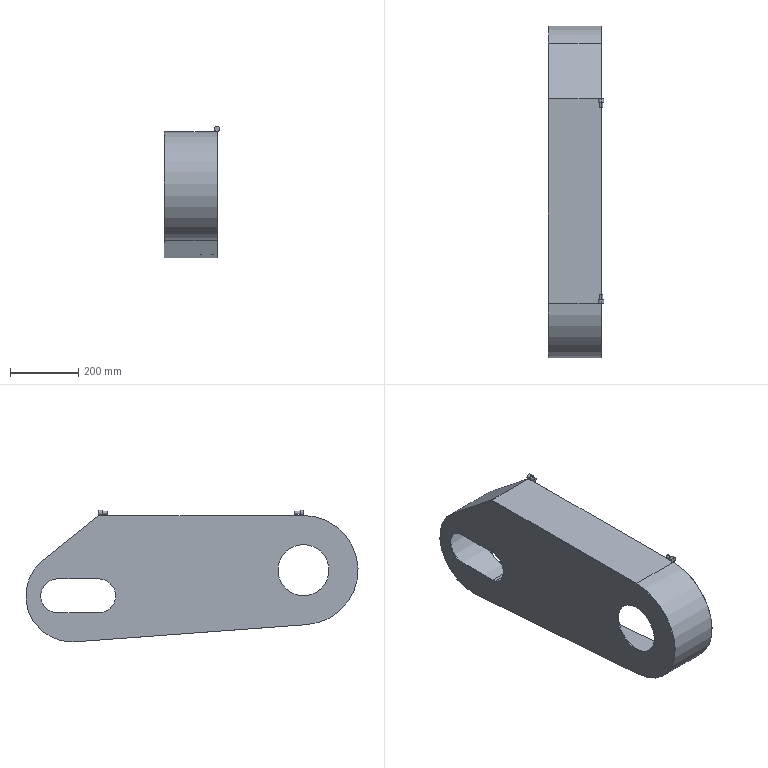Part | SolidWorks | features ICE 7, Extrusion 1, HoleWzd 1, WeldBeadFeat 1, WeldmentFeature 1 | 6 solids | 52 faces | box 163 x 973.632 x 386.5 mm | volume 1244808 mm3 | cylinder 29 | plane 23 | commonest cylinder face diameters 4.2 x8 10 x4 16 x4 270 x4 100 x2 150 x2
STEP:
#1=CARTESIAN_POINT('',(-160.,-325.,-45.));
#2=VERTEX_POINT('',#1);
#3=CARTESIAN_POINT('',(-160.,-325.,105.));
#4=VERTEX_POINT('',#3);
#5=CARTESIAN_POINT('',(-160.,-325.,30.));
#6=DIRECTION('',(-1.,0.,0.));
#7=DIRECTION('',(0.,0.,1.));
#8=AXIS2_PLACEMENT_3D('',#5,#6,#7);
#9=CIRCLE('',#8,75.);
#10=EDGE_CURVE('',#2,#4,#9,.T.);
#11=ORIENTED_EDGE('',*,*,#10,.T.);
#12=CARTESIAN_POINT('',(-158.,-325.,105.));
#13=VERTEX_POINT('',#12);
#14=CARTESIAN_POINT('',(-160.,-325.,105.));
#15=DIRECTION('',(1.,0.,0.));
#16=VECTOR('',#15,1000.);
#17=LINE('',#14,#16);
#18=EDGE_CURVE('',#4,#13,#17,.T.);
#19=ORIENTED_EDGE('',*,*,#18,.T.);
#20=CARTESIAN_POINT('',(-158.,-325.,-45.));
#21=VERTEX_POINT('',#20);
#22=CARTESIAN_POINT('',(-158.,-325.,30.));
#23=DIRECTION('',(-1.,0.,0.));
#24=DIRECTION('',(0.,0.,1.));
#25=AXIS2_PLACEMENT_3D('',#22,#23,#24);
#26=CIRCLE('',#25,75.);
#27=EDGE_CURVE('',#21,#13,#26,.T.);
#28=ORIENTED_EDGE('',*,*,#27,.F.);
#29=CARTESIAN_POINT('',(-160.,-325.,-45.));
#30=DIRECTION('',(1.,0.,0.));
#31=VECTOR('',#30,1000.);
#32=LINE('',#29,#31);
#33=EDGE_CURVE('',#2,#21,#32,.T.);
#34=ORIENTED_EDGE('',*,*,#33,.F.);
#35=EDGE_LOOP('',(#11,#19,#28,#34));
#36=FACE_OUTER_BOUND('',#35,.T.);
#37=CARTESIAN_POINT('',(-160.,-325.,30.));
#38=DIRECTION('',(1.,0.,0.));
#39=DIRECTION('',(0.,0.,-1.));
#40=AXIS2_PLACEMENT_3D('',#37,#38,#39);
#41=CYLINDRICAL_SURFACE('',#40,75.);
#42=ADVANCED_FACE('',(#36),#41,.F.);
#43=CARTESIAN_POINT('',(-160.,353.632,-180.5));
#44=VERTEX_POINT('',#43);
#45=CARTESIAN_POINT('',(-160.,343.627,-180.129));
#46=VERTEX_POINT('',#45);
#47=CARTESIAN_POINT('',(-160.,353.632,-45.5));
#48=DIRECTION('',(-1.,0.,0.));
#49=DIRECTION('',(0.,0.,1.));
#50=AXIS2_PLACEMENT_3D('',#47,#48,#49);
#51=CIRCLE('',#50,135.);
#52=EDGE_CURVE('',#44,#46,#51,.T.);
#53=ORIENTED_EDGE('',*,*,#52,.F.);
#54=CARTESIAN_POINT('',(-158.,353.632,-180.5));
#55=VERTEX_POINT('',#54);
#56=CARTESIAN_POINT('',(-160.,353.632,-180.5));
#57=DIRECTION('',(1.,0.,0.));
#58=VECTOR('',#57,1000.);
#59=LINE('',#56,#58);
#60=EDGE_CURVE('',#44,#55,#59,.T.);
#61=ORIENTED_EDGE('',*,*,#60,.T.);
#62=CARTESIAN_POINT('',(-158.,343.627,-180.129));
#63=VERTEX_POINT('',#62);
#64=CARTESIAN_POINT('',(-158.,353.632,-45.5));
#65=DIRECTION('',(-1.,0.,0.));
#66=DIRECTION('',(0.,0.,1.));
#67=AXIS2_PLACEMENT_3D('',#64,#65,#66);
#68=CIRCLE('',#67,135.);
#69=EDGE_CURVE('',#55,#63,#68,.T.);
#70=ORIENTED_EDGE('',*,*,#69,.T.);
#71=CARTESIAN_POINT('',(-160.,343.627,-180.129));
#72=DIRECTION('',(1.,0.,0.));
#73=VECTOR('',#72,1000.);
#74=LINE('',#71,#73);
#75=EDGE_CURVE('',#46,#63,#74,.T.);
#76=ORIENTED_EDGE('',*,*,#75,.F.);
#77=EDGE_LOOP('',(#53,#61,#70,#76));
#78=FACE_OUTER_BOUND('',#77,.T.);
#79=CARTESIAN_POINT('',(-160.,353.632,-45.5));
#80=DIRECTION('',(1.,0.,0.));
#81=DIRECTION('',(0.,0.,-1.));
#82=AXIS2_PLACEMENT_3D('',#79,#80,#81);
#83=CYLINDRICAL_SURFACE('',#82,135.);
#84=ADVANCED_FACE('',(#78),#83,.T.);
#85=CARTESIAN_POINT('',(-160.,-336.857,-129.56));
#86=VERTEX_POINT('',#85);
#87=CARTESIAN_POINT('',(-160.,-325.,190.));
#88=VERTEX_POINT('',#87);
#89=CARTESIAN_POINT('',(-160.,-325.,30.));
#90=DIRECTION('',(-1.,0.,0.));
#91=DIRECTION('',(0.,0.,1.));
#92=AXIS2_PLACEMENT_3D('',#89,#90,#91);
#93=CIRCLE('',#92,160.);
#94=EDGE_CURVE('',#86,#88,#93,.T.);
#95=ORIENTED_EDGE('',*,*,#94,.T.);
#96=CARTESIAN_POINT('',(-160.,275.,190.));
#97=VERTEX_POINT('',#96);
#98=CARTESIAN_POINT('',(-160.,-325.,190.));
#99=DIRECTION('',(0.,1.,0.));
#100=VECTOR('',#99,1000.);
#101=LINE('',#98,#100);
#102=EDGE_CURVE('',#88,#97,#101,.T.);
#103=ORIENTED_EDGE('',*,*,#102,.T.);
#104=CARTESIAN_POINT('',(-160.,437.851,60.009));
#105=VERTEX_POINT('',#104);
#106=CARTESIAN_POINT('',(-160.,275.,190.));
#107=DIRECTION('',(0.,0.7815,-0.6238));
#108=VECTOR('',#107,1000.);
#109=LINE('',#106,#108);
#110=EDGE_CURVE('',#97,#105,#109,.T.);
#111=ORIENTED_EDGE('',*,*,#110,.T.);
#112=CARTESIAN_POINT('',(-160.,353.632,-45.5));
#113=DIRECTION('',(-1.,0.,0.));
#114=DIRECTION('',(0.,0.,1.));
#115=AXIS2_PLACEMENT_3D('',#112,#113,#114);
#116=CIRCLE('',#115,135.);
#117=EDGE_CURVE('',#105,#44,#116,.T.);
#118=ORIENTED_EDGE('',*,*,#117,.T.);
#119=ORIENTED_EDGE('',*,*,#52,.T.);
#120=CARTESIAN_POINT('',(-160.,343.627,-180.129));
#121=DIRECTION('',(0.,-0.9973,0.07411));
#122=VECTOR('',#121,1000.);
#123=LINE('',#120,#122);
#124=EDGE_CURVE('',#46,#86,#123,.T.);
#125=ORIENTED_EDGE('',*,*,#124,.T.);
#126=EDGE_LOOP('',(#95,#103,#111,#118,#119,#125));
#127=FACE_OUTER_BOUND('',#126,.T.);
#128=ORIENTED_EDGE('',*,*,#10,.F.);
#129=CARTESIAN_POINT('',(-160.,-325.,30.));
#130=DIRECTION('',(-1.,0.,0.));
#131=DIRECTION('',(0.,0.,1.));
#132=AXIS2_PLACEMENT_3D('',#129,#130,#131);
#133=CIRCLE('',#132,75.);
#134=EDGE_CURVE('',#4,#2,#133,.T.);
#135=ORIENTED_EDGE('',*,*,#134,.F.);
#136=EDGE_LOOP('',(#128,#135));
#137=FACE_BOUND('',#136,.T.);
#138=CARTESIAN_POINT('',(-160.,395.,-95.5));
#139=VERTEX_POINT('',#138);
#140=CARTESIAN_POINT('',(-160.,275.,-95.5));
#141=VERTEX_POINT('',#140);
#142=CARTESIAN_POINT('',(-160.,395.,-95.5));
#143=DIRECTION('',(0.,-1.,0.));
#144=VECTOR('',#143,1000.);
#145=LINE('',#142,#144);
#146=EDGE_CURVE('',#139,#141,#145,.T.);
#147=ORIENTED_EDGE('',*,*,#146,.F.);
#148=CARTESIAN_POINT('',(-160.,395.,4.5));
#149=VERTEX_POINT('',#148);
#150=CARTESIAN_POINT('',(-160.,395.,-45.5));
#151=DIRECTION('',(-1.,0.,0.));
#152=DIRECTION('',(0.,0.,1.));
#153=AXIS2_PLACEMENT_3D('',#150,#151,#152);
#154=CIRCLE('',#153,50.);
#155=EDGE_CURVE('',#149,#139,#154,.T.);
#156=ORIENTED_EDGE('',*,*,#155,.F.);
#157=CARTESIAN_POINT('',(-160.,275.,4.5));
#158=VERTEX_POINT('',#157);
#159=CARTESIAN_POINT('',(-160.,395.,4.5));
#160=DIRECTION('',(0.,1.,0.));
#161=VECTOR('',#160,1000.);
#162=LINE('',#159,#161);
#163=EDGE_CURVE('',#158,#149,#162,.T.);
#164=ORIENTED_EDGE('',*,*,#163,.F.);
#165=CARTESIAN_POINT('',(-160.,275.,-45.5));
#166=DIRECTION('',(-1.,0.,0.));
#167=DIRECTION('',(0.,0.,1.));
#168=AXIS2_PLACEMENT_3D('',#165,#166,#167);
#169=CIRCLE('',#168,50.);
#170=EDGE_CURVE('',#141,#158,#169,.T.);
#171=ORIENTED_EDGE('',*,*,#170,.F.);
#172=EDGE_LOOP('',(#147,#156,#164,#171));
#173=FACE_BOUND('',#172,.T.);
#174=CARTESIAN_POINT('',(-160.,-325.,30.));
#175=DIRECTION('',(-1.,0.,0.));
#176=DIRECTION('',(0.,0.,1.));
#177=AXIS2_PLACEMENT_3D('',#174,#175,#176);
#178=PLANE('',#177);
#179=ADVANCED_FACE('',(#127,#137,#173),#178,.T.);
#180=ORIENTED_EDGE('',*,*,#27,.T.);
#181=CARTESIAN_POINT('',(-158.,-325.,30.));
#182=DIRECTION('',(-1.,0.,0.));
#183=DIRECTION('',(0.,0.,1.));
#184=AXIS2_PLACEMENT_3D('',#181,#182,#183);
#185=CIRCLE('',#184,75.);
#186=EDGE_CURVE('',#13,#21,#185,.T.);
#187=ORIENTED_EDGE('',*,*,#186,.T.);
#188=EDGE_LOOP('',(#180,#187));
#189=FACE_BOUND('',#188,.T.);
#190=CARTESIAN_POINT('',(-158.,-336.857,-129.56));
#191=VERTEX_POINT('',#190);
#192=CARTESIAN_POINT('',(-158.,-325.,190.));
#193=VERTEX_POINT('',#192);
#194=CARTESIAN_POINT('',(-158.,-325.,30.));
#195=DIRECTION('',(-1.,0.,0.));
#196=DIRECTION('',(0.,0.,1.));
#197=AXIS2_PLACEMENT_3D('',#194,#195,#196);
#198=CIRCLE('',#197,160.);
#199=EDGE_CURVE('',#191,#193,#198,.T.);
#200=ORIENTED_EDGE('',*,*,#199,.F.);
#201=CARTESIAN_POINT('',(-158.,343.627,-180.129));
#202=DIRECTION('',(0.,-0.9973,0.07411));
#203=VECTOR('',#202,1000.);
#204=LINE('',#201,#203);
#205=EDGE_CURVE('',#63,#191,#204,.T.);
#206=ORIENTED_EDGE('',*,*,#205,.F.);
#207=ORIENTED_EDGE('',*,*,#69,.F.);
#208=CARTESIAN_POINT('',(-158.,437.851,60.009));
#209=VERTEX_POINT('',#208);
#210=CARTESIAN_POINT('',(-158.,353.632,-45.5));
#211=DIRECTION('',(-1.,0.,0.));
#212=DIRECTION('',(0.,0.,1.));
#213=AXIS2_PLACEMENT_3D('',#210,#211,#212);
#214=CIRCLE('',#213,135.);
#215=EDGE_CURVE('',#209,#55,#214,.T.);
#216=ORIENTED_EDGE('',*,*,#215,.F.);
#217=CARTESIAN_POINT('',(-158.,275.,190.));
#218=VERTEX_POINT('',#217);
#219=CARTESIAN_POINT('',(-158.,275.,190.));
#220=DIRECTION('',(0.,0.7815,-0.6238));
#221=VECTOR('',#220,1000.);
#222=LINE('',#219,#221);
#223=EDGE_CURVE('',#218,#209,#222,.T.);
#224=ORIENTED_EDGE('',*,*,#223,.F.);
#225=CARTESIAN_POINT('',(-158.,-325.,190.));
#226=DIRECTION('',(0.,1.,0.));
#227=VECTOR('',#226,1000.);
#228=LINE('',#225,#227);
#229=EDGE_CURVE('',#193,#218,#228,.T.);
#230=ORIENTED_EDGE('',*,*,#229,.F.);
#231=EDGE_LOOP('',(#200,#206,#207,#216,#224,#230));
#232=FACE_OUTER_BOUND('',#231,.T.);
#233=CARTESIAN_POINT('',(-158.,395.,4.5));
#234=VERTEX_POINT('',#233);
#235=CARTESIAN_POINT('',(-158.,395.,-95.5));
#236=VERTEX_POINT('',#235);
#237=CARTESIAN_POINT('',(-158.,395.,-45.5));
#238=DIRECTION('',(-1.,0.,0.));
#239=DIRECTION('',(0.,0.,1.));
#240=AXIS2_PLACEMENT_3D('',#237,#238,#239);
#241=CIRCLE('',#240,50.);
#242=EDGE_CURVE('',#234,#236,#241,.T.);
#243=ORIENTED_EDGE('',*,*,#242,.T.);
#244=CARTESIAN_POINT('',(-158.,275.,-95.5));
#245=VERTEX_POINT('',#244);
#246=CARTESIAN_POINT('',(-158.,395.,-95.5));
#247=DIRECTION('',(0.,-1.,0.));
#248=VECTOR('',#247,1000.);
#249=LINE('',#246,#248);
#250=EDGE_CURVE('',#236,#245,#249,.T.);
#251=ORIENTED_EDGE('',*,*,#250,.T.);
#252=CARTESIAN_POINT('',(-158.,275.,4.5));
#253=VERTEX_POINT('',#252);
#254=CARTESIAN_POINT('',(-158.,275.,-45.5));
#255=DIRECTION('',(-1.,0.,0.));
#256=DIRECTION('',(0.,0.,1.));
#257=AXIS2_PLACEMENT_3D('',#254,#255,#256);
#258=CIRCLE('',#257,50.);
#259=EDGE_CURVE('',#245,#253,#258,.T.);
#260=ORIENTED_EDGE('',*,*,#259,.T.);
#261=CARTESIAN_POINT('',(-158.,395.,4.5));
#262=DIRECTION('',(0.,1.,0.));
#263=VECTOR('',#262,1000.);
#264=LINE('',#261,#263);
#265=EDGE_CURVE('',#253,#234,#264,.T.);
#266=ORIENTED_EDGE('',*,*,#265,.T.);
#267=EDGE_LOOP('',(#243,#251,#260,#266));
#268=FACE_BOUND('',#267,.T.);
#269=CARTESIAN_POINT('',(-158.,-325.,30.));
#270=DIRECTION('',(-1.,0.,0.));
#271=DIRECTION('',(0.,0.,1.));
#272=AXIS2_PLACEMENT_3D('',#269,#270,#271);
#273=PLANE('',#272);
#274=ADVANCED_FACE('',(#189,#232,#268),#273,.F.);
#275=ORIENTED_EDGE('',*,*,#199,.T.);
#276=CARTESIAN_POINT('',(-160.,-325.,190.));
#277=DIRECTION('',(1.,0.,0.));
#278=VECTOR('',#277,1000.);
#279=LINE('',#276,#278);
#280=EDGE_CURVE('',#88,#193,#279,.T.);
#281=ORIENTED_EDGE('',*,*,#280,.F.);
#282=ORIENTED_EDGE('',*,*,#94,.F.);
#283=CARTESIAN_POINT('',(-160.,-336.857,-129.56));
#284=DIRECTION('',(1.,0.,0.));
#285=VECTOR('',#284,1000.);
#286=LINE('',#283,#285);
#287=EDGE_CURVE('',#86,#191,#286,.T.);
#288=ORIENTED_EDGE('',*,*,#287,.T.);
#289=EDGE_LOOP('',(#275,#281,#282,#288));
#290=FACE_OUTER_BOUND('',#289,.T.);
#291=CARTESIAN_POINT('',(-160.,-325.,30.));
#292=DIRECTION('',(1.,0.,0.));
#293=DIRECTION('',(0.,0.,-1.));
#294=AXIS2_PLACEMENT_3D('',#291,#292,#293);
#295=CYLINDRICAL_SURFACE('',#294,160.);
#296=ADVANCED_FACE('',(#290),#295,.T.);
#297=ORIENTED_EDGE('',*,*,#229,.T.);
#298=CARTESIAN_POINT('',(-160.,275.,190.));
#299=DIRECTION('',(1.,0.,0.));
#300=VECTOR('',#299,1000.);
#301=LINE('',#298,#300);
#302=EDGE_CURVE('',#97,#218,#301,.T.);
#303=ORIENTED_EDGE('',*,*,#302,.F.);
#304=ORIENTED_EDGE('',*,*,#102,.F.);
#305=ORIENTED_EDGE('',*,*,#280,.T.);
#306=EDGE_LOOP('',(#297,#303,#304,#305));
#307=FACE_OUTER_BOUND('',#306,.T.);
#308=CARTESIAN_POINT('',(-160.,-325.,190.));
#309=DIRECTION('',(0.,0.,-1.));
#310=DIRECTION('',(0.,1.,0.));
#311=AXIS2_PLACEMENT_3D('',#308,#309,#310);
#312=PLANE('',#311);
#313=ADVANCED_FACE('',(#307),#312,.F.);
#314=ORIENTED_EDGE('',*,*,#223,.T.);
#315=CARTESIAN_POINT('',(-160.,437.851,60.009));
#316=DIRECTION('',(1.,0.,0.));
#317=VECTOR('',#316,1000.);
#318=LINE('',#315,#317);
#319=EDGE_CURVE('',#105,#209,#318,.T.);
#320=ORIENTED_EDGE('',*,*,#319,.F.);
#321=ORIENTED_EDGE('',*,*,#110,.F.);
#322=ORIENTED_EDGE('',*,*,#302,.T.);
#323=EDGE_LOOP('',(#314,#320,#321,#322));
#324=FACE_OUTER_BOUND('',#323,.T.);
#325=CARTESIAN_POINT('',(-160.,275.,190.));
#326=DIRECTION('',(0.,-0.6238,-0.7815));
#327=DIRECTION('',(0.,0.7815,-0.6238));
#328=AXIS2_PLACEMENT_3D('',#325,#326,#327);
#329=PLANE('',#328);
#330=ADVANCED_FACE('',(#324),#329,.F.);
#331=ORIENTED_EDGE('',*,*,#60,.F.);
#332=ORIENTED_EDGE('',*,*,#117,.F.);
#333=ORIENTED_EDGE('',*,*,#319,.T.);
#334=ORIENTED_EDGE('',*,*,#215,.T.);
#335=EDGE_LOOP('',(#331,#332,#333,#334));
#336=FACE_OUTER_BOUND('',#335,.T.);
#337=CARTESIAN_POINT('',(-160.,353.632,-45.5));
#338=DIRECTION('',(1.,0.,0.));
#339=DIRECTION('',(0.,0.,-1.));
#340=AXIS2_PLACEMENT_3D('',#337,#338,#339);
#341=CYLINDRICAL_SURFACE('',#340,135.);
#342=ADVANCED_FACE('',(#336),#341,.T.);
#343=ORIENTED_EDGE('',*,*,#205,.T.);
#344=ORIENTED_EDGE('',*,*,#287,.F.);
#345=ORIENTED_EDGE('',*,*,#124,.F.);
#346=ORIENTED_EDGE('',*,*,#75,.T.);
#347=EDGE_LOOP('',(#343,#344,#345,#346));
#348=FACE_OUTER_BOUND('',#347,.T.);
#349=CARTESIAN_POINT('',(-160.,343.627,-180.129));
#350=DIRECTION('',(0.,0.07411,0.9973));
#351=DIRECTION('',(0.,-0.9973,0.07411));
#352=AXIS2_PLACEMENT_3D('',#349,#350,#351);
#353=PLANE('',#352);
#354=ADVANCED_FACE('',(#348),#353,.F.);
#355=ORIENTED_EDGE('',*,*,#18,.F.);
#356=ORIENTED_EDGE('',*,*,#134,.T.);
#357=ORIENTED_EDGE('',*,*,#33,.T.);
#358=ORIENTED_EDGE('',*,*,#186,.F.);
#359=EDGE_LOOP('',(#355,#356,#357,#358));
#360=FACE_OUTER_BOUND('',#359,.T.);
#361=CARTESIAN_POINT('',(-160.,-325.,30.));
#362=DIRECTION('',(1.,0.,0.));
#363=DIRECTION('',(0.,0.,-1.));
#364=AXIS2_PLACEMENT_3D('',#361,#362,#363);
#365=CYLINDRICAL_SURFACE('',#364,75.);
#366=ADVANCED_FACE('',(#360),#365,.F.);
#367=ORIENTED_EDGE('',*,*,#242,.F.);
#368=CARTESIAN_POINT('',(-160.,395.,4.5));
#369=DIRECTION('',(1.,0.,0.));
#370=VECTOR('',#369,1000.);
#371=LINE('',#368,#370);
#372=EDGE_CURVE('',#149,#234,#371,.T.);
#373=ORIENTED_EDGE('',*,*,#372,.F.);
#374=ORIENTED_EDGE('',*,*,#155,.T.);
#375=CARTESIAN_POINT('',(-160.,395.,-95.5));
#376=DIRECTION('',(1.,0.,0.));
#377=VECTOR('',#376,1000.);
#378=LINE('',#375,#377);
#379=EDGE_CURVE('',#139,#236,#378,.T.);
#380=ORIENTED_EDGE('',*,*,#379,.T.);
#381=EDGE_LOOP('',(#367,#373,#374,#380));
#382=FACE_OUTER_BOUND('',#381,.T.);
#383=CARTESIAN_POINT('',(-160.,395.,-45.5));
#384=DIRECTION('',(1.,0.,0.));
#385=DIRECTION('',(0.,0.,-1.));
#386=AXIS2_PLACEMENT_3D('',#383,#384,#385);
#387=CYLINDRICAL_SURFACE('',#386,50.);
#388=ADVANCED_FACE('',(#382),#387,.F.);
#389=ORIENTED_EDGE('',*,*,#250,.F.);
#390=ORIENTED_EDGE('',*,*,#379,.F.);
#391=ORIENTED_EDGE('',*,*,#146,.T.);
#392=CARTESIAN_POINT('',(-160.,275.,-95.5));
#393=DIRECTION('',(1.,0.,0.));
#394=VECTOR('',#393,1000.);
#395=LINE('',#392,#394);
#396=EDGE_CURVE('',#141,#245,#395,.T.);
#397=ORIENTED_EDGE('',*,*,#396,.T.);
#398=EDGE_LOOP('',(#389,#390,#391,#397));
#399=FACE_OUTER_BOUND('',#398,.T.);
#400=CARTESIAN_POINT('',(-160.,395.,-95.5));
#401=DIRECTION('',(0.,0.,1.));
#402=DIRECTION('',(0.,-1.,0.));
#403=AXIS2_PLACEMENT_3D('',#400,#401,#402);
#404=PLANE('',#403);
#405=ADVANCED_FACE('',(#399),#404,.T.);
#406=ORIENTED_EDGE('',*,*,#259,.F.);
#407=ORIENTED_EDGE('',*,*,#396,.F.);
#408=ORIENTED_EDGE('',*,*,#170,.T.);
#409=CARTESIAN_POINT('',(-160.,275.,4.5));
#410=DIRECTION('',(1.,0.,0.));
#411=VECTOR('',#410,1000.);
#412=LINE('',#409,#411);
#413=EDGE_CURVE('',#158,#253,#412,.T.);
#414=ORIENTED_EDGE('',*,*,#413,.T.);
#415=EDGE_LOOP('',(#406,#407,#408,#414));
#416=FACE_OUTER_BOUND('',#415,.T.);
#417=CARTESIAN_POINT('',(-160.,275.,-45.5));
#418=DIRECTION('',(1.,0.,0.));
#419=DIRECTION('',(0.,0.,-1.));
#420=AXIS2_PLACEMENT_3D('',#417,#418,#419);
#421=CYLINDRICAL_SURFACE('',#420,50.);
#422=ADVANCED_FACE('',(#416),#421,.F.);
#423=ORIENTED_EDGE('',*,*,#265,.F.);
#424=ORIENTED_EDGE('',*,*,#413,.F.);
#425=ORIENTED_EDGE('',*,*,#163,.T.);
#426=ORIENTED_EDGE('',*,*,#372,.T.);
#427=EDGE_LOOP('',(#423,#424,#425,#426));
#428=FACE_OUTER_BOUND('',#427,.T.);
#429=CARTESIAN_POINT('',(-160.,395.,4.5));
#430=DIRECTION('',(0.,0.,-1.));
#431=DIRECTION('',(0.,1.,0.));
#432=AXIS2_PLACEMENT_3D('',#429,#430,#431);
#433=PLANE('',#432);
#434=ADVANCED_FACE('',(#428),#433,.T.);
#435=CLOSED_SHELL('',(#42,#84,#179,#274,#296,#313,#330,#342,#354,#366,#388,#405,#422,#434));
#436=MANIFOLD_SOLID_BREP('',#435);
#437=CARTESIAN_POINT('',(-5.,-315.,206.));
#438=VERTEX_POINT('',#437);
#439=CARTESIAN_POINT('',(-5.,-315.,190.));
#440=VERTEX_POINT('',#439);
#441=CARTESIAN_POINT('',(-5.,-315.,198.));
#442=DIRECTION('',(0.,1.,0.));
#443=DIRECTION('',(0.,0.,1.));
#444=AXIS2_PLACEMENT_3D('',#441,#442,#443);
#445=CIRCLE('',#444,8.);
#446=EDGE_CURVE('',#438,#440,#445,.T.);
#447=ORIENTED_EDGE('',*,*,#446,.F.);
#448=CARTESIAN_POINT('',(-5.,-325.,206.));
#449=VERTEX_POINT('',#448);
#450=CARTESIAN_POINT('',(-5.,-315.,206.));
#451=DIRECTION('',(0.,-1.,0.));
#452=VECTOR('',#451,1000.);
#453=LINE('',#450,#452);
#454=EDGE_CURVE('',#438,#449,#453,.T.);
#455=ORIENTED_EDGE('',*,*,#454,.T.);
#456=CARTESIAN_POINT('',(-5.,-325.,190.));
#457=VERTEX_POINT('',#456);
#458=CARTESIAN_POINT('',(-5.,-325.,198.));
#459=DIRECTION('',(0.,1.,0.));
#460=DIRECTION('',(0.,0.,1.));
#461=AXIS2_PLACEMENT_3D('',#458,#459,#460);
#462=CIRCLE('',#461,8.);
#463=EDGE_CURVE('',#449,#457,#462,.T.);
#464=ORIENTED_EDGE('',*,*,#463,.T.);
#465=CARTESIAN_POINT('',(-5.,-315.,190.));
#466=DIRECTION('',(0.,-1.,0.));
#467=VECTOR('',#466,1000.);
#468=LINE('',#465,#467);
#469=EDGE_CURVE('',#440,#457,#468,.T.);
#470=ORIENTED_EDGE('',*,*,#469,.F.);
#471=EDGE_LOOP('',(#447,#455,#464,#470));
#472=FACE_OUTER_BOUND('',#471,.T.);
#473=CARTESIAN_POINT('',(-5.,-315.,198.));
#474=DIRECTION('',(0.,-1.,0.));
#475=DIRECTION('',(0.,0.,-1.));
#476=AXIS2_PLACEMENT_3D('',#473,#474,#475);
#477=CYLINDRICAL_SURFACE('',#476,8.);
#478=ADVANCED_FACE('',(#472),#477,.T.);
#479=ORIENTED_EDGE('',*,*,#454,.F.);
#480=CARTESIAN_POINT('',(-5.,-315.,198.));
#481=DIRECTION('',(0.,1.,0.));
#482=DIRECTION('',(0.,0.,1.));
#483=AXIS2_PLACEMENT_3D('',#480,#481,#482);
#484=CIRCLE('',#483,8.);
#485=EDGE_CURVE('',#440,#438,#484,.T.);
#486=ORIENTED_EDGE('',*,*,#485,.F.);
#487=ORIENTED_EDGE('',*,*,#469,.T.);
#488=CARTESIAN_POINT('',(-5.,-325.,198.));
#489=DIRECTION('',(0.,1.,0.));
#490=DIRECTION('',(0.,0.,1.));
#491=AXIS2_PLACEMENT_3D('',#488,#489,#490);
#492=CIRCLE('',#491,8.);
#493=EDGE_CURVE('',#457,#449,#492,.T.);
#494=ORIENTED_EDGE('',*,*,#493,.T.);
#495=EDGE_LOOP('',(#479,#486,#487,#494));
#496=FACE_OUTER_BOUND('',#495,.T.);
#497=CARTESIAN_POINT('',(-5.,-315.,198.));
#498=DIRECTION('',(0.,-1.,0.));
#499=DIRECTION('',(0.,0.,-1.));
#500=AXIS2_PLACEMENT_3D('',#497,#498,#499);
#501=CYLINDRICAL_SURFACE('',#500,8.);
#502=ADVANCED_FACE('',(#496),#501,.T.);
#503=ORIENTED_EDGE('',*,*,#485,.T.);
#504=ORIENTED_EDGE('',*,*,#446,.T.);
#505=EDGE_LOOP('',(#503,#504));
#506=FACE_OUTER_BOUND('',#505,.T.);
#507=CARTESIAN_POINT('',(-5.,-315.,198.));
#508=DIRECTION('',(0.,1.,0.));
#509=DIRECTION('',(0.,0.,1.));
#510=AXIS2_PLACEMENT_3D('',#507,#508,#509);
#511=PLANE('',#510);
#512=ADVANCED_FACE('',(#506),#511,.T.);
#513=ORIENTED_EDGE('',*,*,#493,.F.);
#514=ORIENTED_EDGE('',*,*,#463,.F.);
#515=EDGE_LOOP('',(#513,#514));
#516=FACE_OUTER_BOUND('',#515,.T.);
#517=CARTESIAN_POINT('',(-5.,-325.,198.));
#518=DIRECTION('',(0.,1.,0.));
#519=DIRECTION('',(0.,0.,1.));
#520=AXIS2_PLACEMENT_3D('',#517,#518,#519);
#521=PLANE('',#520);
#522=ADVANCED_FACE('',(#516),#521,.F.);
#523=CLOSED_SHELL('',(#478,#502,#512,#522));
#524=MANIFOLD_SOLID_BREP('',#523);
#525=CARTESIAN_POINT('',(-5.,-300.,203.));
#526=VERTEX_POINT('',#525);
#527=CARTESIAN_POINT('',(-5.,-300.,193.));
#528=VERTEX_POINT('',#527);
#529=CARTESIAN_POINT('',(-5.,-300.,198.));
#530=DIRECTION('',(0.,1.,0.));
#531=DIRECTION('',(0.,0.,1.));
#532=AXIS2_PLACEMENT_3D('',#529,#530,#531);
#533=CIRCLE('',#532,5.);
#534=EDGE_CURVE('',#526,#528,#533,.T.);
#535=ORIENTED_EDGE('',*,*,#534,.F.);
#536=CARTESIAN_POINT('',(-5.,-315.,203.));
#537=VERTEX_POINT('',#536);
#538=CARTESIAN_POINT('',(-5.,-300.,203.));
#539=DIRECTION('',(0.,-1.,0.));
#540=VECTOR('',#539,1000.);
#541=LINE('',#538,#540);
#542=EDGE_CURVE('',#526,#537,#541,.T.);
#543=ORIENTED_EDGE('',*,*,#542,.T.);
#544=CARTESIAN_POINT('',(-5.,-315.,193.));
#545=VERTEX_POINT('',#544);
#546=CARTESIAN_POINT('',(-5.,-315.,198.));
#547=DIRECTION('',(0.,1.,0.));
#548=DIRECTION('',(0.,0.,1.));
#549=AXIS2_PLACEMENT_3D('',#546,#547,#548);
#550=CIRCLE('',#549,5.);
#551=EDGE_CURVE('',#537,#545,#550,.T.);
#552=ORIENTED_EDGE('',*,*,#551,.T.);
#553=CARTESIAN_POINT('',(-5.,-300.,193.));
#554=DIRECTION('',(0.,-1.,0.));
#555=VECTOR('',#554,1000.);
#556=LINE('',#553,#555);
#557=EDGE_CURVE('',#528,#545,#556,.T.);
#558=ORIENTED_EDGE('',*,*,#557,.F.);
#559=EDGE_LOOP('',(#535,#543,#552,#558));
#560=FACE_OUTER_BOUND('',#559,.T.);
#561=CARTESIAN_POINT('',(-5.,-300.,198.));
#562=DIRECTION('',(0.,-1.,0.));
#563=DIRECTION('',(0.,0.,-1.));
#564=AXIS2_PLACEMENT_3D('',#561,#562,#563);
#565=CYLINDRICAL_SURFACE('',#564,5.);
#566=ADVANCED_FACE('',(#560),#565,.T.);
#567=ORIENTED_EDGE('',*,*,#542,.F.);
#568=CARTESIAN_POINT('',(-5.,-300.,198.));
#569=DIRECTION('',(0.,1.,0.));
#570=DIRECTION('',(0.,0.,1.));
#571=AXIS2_PLACEMENT_3D('',#568,#569,#570);
#572=CIRCLE('',#571,5.);
#573=EDGE_CURVE('',#528,#526,#572,.T.);
#574=ORIENTED_EDGE('',*,*,#573,.F.);
#575=ORIENTED_EDGE('',*,*,#557,.T.);
#576=CARTESIAN_POINT('',(-5.,-315.,198.));
#577=DIRECTION('',(0.,1.,0.));
#578=DIRECTION('',(0.,0.,1.));
#579=AXIS2_PLACEMENT_3D('',#576,#577,#578);
#580=CIRCLE('',#579,5.);
#581=EDGE_CURVE('',#545,#537,#580,.T.);
#582=ORIENTED_EDGE('',*,*,#581,.T.);
#583=EDGE_LOOP('',(#567,#574,#575,#582));
#584=FACE_OUTER_BOUND('',#583,.T.);
#585=CARTESIAN_POINT('',(-5.,-300.,198.));
#586=DIRECTION('',(0.,-1.,0.));
#587=DIRECTION('',(0.,0.,-1.));
#588=AXIS2_PLACEMENT_3D('',#585,#586,#587);
#589=CYLINDRICAL_SURFACE('',#588,5.);
#590=ADVANCED_FACE('',(#584),#589,.T.);
#591=ORIENTED_EDGE('',*,*,#573,.T.);
#592=ORIENTED_EDGE('',*,*,#534,.T.);
#593=EDGE_LOOP('',(#591,#592));
#594=FACE_OUTER_BOUND('',#593,.T.);
#595=CARTESIAN_POINT('',(-5.,-300.,198.));
#596=DIRECTION('',(0.,1.,0.));
#597=DIRECTION('',(0.,0.,1.));
#598=AXIS2_PLACEMENT_3D('',#595,#596,#597);
#599=PLANE('',#598);
#600=ADVANCED_FACE('',(#594),#599,.T.);
#601=ORIENTED_EDGE('',*,*,#581,.F.);
#602=ORIENTED_EDGE('',*,*,#551,.F.);
#603=EDGE_LOOP('',(#601,#602));
#604=FACE_OUTER_BOUND('',#603,.T.);
#605=CARTESIAN_POINT('',(-5.,-315.,198.));
#606=DIRECTION('',(0.,1.,0.));
#607=DIRECTION('',(0.,0.,1.));
#608=AXIS2_PLACEMENT_3D('',#605,#606,#607);
#609=PLANE('',#608);
#610=ADVANCED_FACE('',(#604),#609,.F.);
#611=CLOSED_SHELL('',(#566,#590,#600,#610));
#612=MANIFOLD_SOLID_BREP('',#611);
#613=CARTESIAN_POINT('',(-5.,264.3,206.));
#614=VERTEX_POINT('',#613);
#615=CARTESIAN_POINT('',(-5.,264.3,190.));
#616=VERTEX_POINT('',#615);
#617=CARTESIAN_POINT('',(-5.,264.3,198.));
#618=DIRECTION('',(0.,1.,0.));
#619=DIRECTION('',(0.,0.,1.));
#620=AXIS2_PLACEMENT_3D('',#617,#618,#619);
#621=CIRCLE('',#620,8.);
#622=EDGE_CURVE('',#614,#616,#621,.T.);
#623=ORIENTED_EDGE('',*,*,#622,.T.);
#624=CARTESIAN_POINT('',(-5.,274.3,190.));
#625=VERTEX_POINT('',#624);
#626=CARTESIAN_POINT('',(-5.,264.3,190.));
#627=DIRECTION('',(0.,1.,0.));
#628=VECTOR('',#627,1000.);
#629=LINE('',#626,#628);
#630=EDGE_CURVE('',#616,#625,#629,.T.);
#631=ORIENTED_EDGE('',*,*,#630,.T.);
#632=CARTESIAN_POINT('',(-5.,274.3,206.));
#633=VERTEX_POINT('',#632);
#634=CARTESIAN_POINT('',(-5.,274.3,198.));
#635=DIRECTION('',(0.,1.,0.));
#636=DIRECTION('',(0.,0.,1.));
#637=AXIS2_PLACEMENT_3D('',#634,#635,#636);
#638=CIRCLE('',#637,8.);
#639=EDGE_CURVE('',#633,#625,#638,.T.);
#640=ORIENTED_EDGE('',*,*,#639,.F.);
#641=CARTESIAN_POINT('',(-5.,264.3,206.));
#642=DIRECTION('',(0.,1.,0.));
#643=VECTOR('',#642,1000.);
#644=LINE('',#641,#643);
#645=EDGE_CURVE('',#614,#633,#644,.T.);
#646=ORIENTED_EDGE('',*,*,#645,.F.);
#647=EDGE_LOOP('',(#623,#631,#640,#646));
#648=FACE_OUTER_BOUND('',#647,.T.);
#649=CARTESIAN_POINT('',(-5.,264.3,198.));
#650=DIRECTION('',(0.,1.,0.));
#651=DIRECTION('',(0.,0.,1.));
#652=AXIS2_PLACEMENT_3D('',#649,#650,#651);
#653=CYLINDRICAL_SURFACE('',#652,8.);
#654=ADVANCED_FACE('',(#648),#653,.T.);
#655=ORIENTED_EDGE('',*,*,#630,.F.);
#656=CARTESIAN_POINT('',(-5.,264.3,198.));
#657=DIRECTION('',(0.,1.,0.));
#658=DIRECTION('',(0.,0.,1.));
#659=AXIS2_PLACEMENT_3D('',#656,#657,#658);
#660=CIRCLE('',#659,8.);
#661=EDGE_CURVE('',#616,#614,#660,.T.);
#662=ORIENTED_EDGE('',*,*,#661,.T.);
#663=ORIENTED_EDGE('',*,*,#645,.T.);
#664=CARTESIAN_POINT('',(-5.,274.3,198.));
#665=DIRECTION('',(0.,1.,0.));
#666=DIRECTION('',(0.,0.,1.));
#667=AXIS2_PLACEMENT_3D('',#664,#665,#666);
#668=CIRCLE('',#667,8.);
#669=EDGE_CURVE('',#625,#633,#668,.T.);
#670=ORIENTED_EDGE('',*,*,#669,.F.);
#671=EDGE_LOOP('',(#655,#662,#663,#670));
#672=FACE_OUTER_BOUND('',#671,.T.);
#673=CARTESIAN_POINT('',(-5.,264.3,198.));
#674=DIRECTION('',(0.,1.,0.));
#675=DIRECTION('',(0.,0.,1.));
#676=AXIS2_PLACEMENT_3D('',#673,#674,#675);
#677=CYLINDRICAL_SURFACE('',#676,8.);
#678=ADVANCED_FACE('',(#672),#677,.T.);
#679=ORIENTED_EDGE('',*,*,#622,.F.);
#680=ORIENTED_EDGE('',*,*,#661,.F.);
#681=EDGE_LOOP('',(#679,#680));
#682=FACE_OUTER_BOUND('',#681,.T.);
#683=CARTESIAN_POINT('',(-5.,264.3,198.));
#684=DIRECTION('',(0.,1.,0.));
#685=DIRECTION('',(0.,0.,1.));
#686=AXIS2_PLACEMENT_3D('',#683,#684,#685);
#687=PLANE('',#686);
#688=ADVANCED_FACE('',(#682),#687,.F.);
#689=ORIENTED_EDGE('',*,*,#639,.T.);
#690=ORIENTED_EDGE('',*,*,#669,.T.);
#691=EDGE_LOOP('',(#689,#690));
#692=FACE_OUTER_BOUND('',#691,.T.);
#693=CARTESIAN_POINT('',(-5.,274.3,198.));
#694=DIRECTION('',(0.,1.,0.));
#695=DIRECTION('',(0.,0.,1.));
#696=AXIS2_PLACEMENT_3D('',#693,#694,#695);
#697=PLANE('',#696);
#698=ADVANCED_FACE('',(#692),#697,.T.);
#699=CLOSED_SHELL('',(#654,#678,#688,#698));
#700=MANIFOLD_SOLID_BREP('',#699);
#701=CARTESIAN_POINT('',(-5.,249.3,193.));
#702=VERTEX_POINT('',#701);
#703=CARTESIAN_POINT('',(-5.,249.3,203.));
#704=VERTEX_POINT('',#703);
#705=CARTESIAN_POINT('',(-5.,249.3,198.));
#706=DIRECTION('',(0.,-1.,0.));
#707=DIRECTION('',(0.,0.,-1.));
#708=AXIS2_PLACEMENT_3D('',#705,#706,#707);
#709=CIRCLE('',#708,5.);
#710=EDGE_CURVE('',#702,#704,#709,.T.);
#711=ORIENTED_EDGE('',*,*,#710,.F.);
#712=CARTESIAN_POINT('',(-5.,264.3,193.));
#713=VERTEX_POINT('',#712);
#714=CARTESIAN_POINT('',(-5.,249.3,193.));
#715=DIRECTION('',(0.,1.,0.));
#716=VECTOR('',#715,1000.);
#717=LINE('',#714,#716);
#718=EDGE_CURVE('',#702,#713,#717,.T.);
#719=ORIENTED_EDGE('',*,*,#718,.T.);
#720=CARTESIAN_POINT('',(-5.,264.3,203.));
#721=VERTEX_POINT('',#720);
#722=CARTESIAN_POINT('',(-5.,264.3,198.));
#723=DIRECTION('',(0.,-1.,0.));
#724=DIRECTION('',(0.,0.,-1.));
#725=AXIS2_PLACEMENT_3D('',#722,#723,#724);
#726=CIRCLE('',#725,5.);
#727=EDGE_CURVE('',#713,#721,#726,.T.);
#728=ORIENTED_EDGE('',*,*,#727,.T.);
#729=CARTESIAN_POINT('',(-5.,249.3,203.));
#730=DIRECTION('',(0.,1.,0.));
#731=VECTOR('',#730,1000.);
#732=LINE('',#729,#731);
#733=EDGE_CURVE('',#704,#721,#732,.T.);
#734=ORIENTED_EDGE('',*,*,#733,.F.);
#735=EDGE_LOOP('',(#711,#719,#728,#734));
#736=FACE_OUTER_BOUND('',#735,.T.);
#737=CARTESIAN_POINT('',(-5.,249.3,198.));
#738=DIRECTION('',(0.,1.,0.));
#739=DIRECTION('',(0.,0.,1.));
#740=AXIS2_PLACEMENT_3D('',#737,#738,#739);
#741=CYLINDRICAL_SURFACE('',#740,5.);
#742=ADVANCED_FACE('',(#736),#741,.T.);
#743=ORIENTED_EDGE('',*,*,#718,.F.);
#744=CARTESIAN_POINT('',(-5.,249.3,198.));
#745=DIRECTION('',(0.,-1.,0.));
#746=DIRECTION('',(0.,0.,-1.));
#747=AXIS2_PLACEMENT_3D('',#744,#745,#746);
#748=CIRCLE('',#747,5.);
#749=EDGE_CURVE('',#704,#702,#748,.T.);
#750=ORIENTED_EDGE('',*,*,#749,.F.);
#751=ORIENTED_EDGE('',*,*,#733,.T.);
#752=CARTESIAN_POINT('',(-5.,264.3,198.));
#753=DIRECTION('',(0.,-1.,0.));
#754=DIRECTION('',(0.,0.,-1.));
#755=AXIS2_PLACEMENT_3D('',#752,#753,#754);
#756=CIRCLE('',#755,5.);
#757=EDGE_CURVE('',#721,#713,#756,.T.);
#758=ORIENTED_EDGE('',*,*,#757,.T.);
#759=EDGE_LOOP('',(#743,#750,#751,#758));
#760=FACE_OUTER_BOUND('',#759,.T.);
#761=CARTESIAN_POINT('',(-5.,249.3,198.));
#762=DIRECTION('',(0.,1.,0.));
#763=DIRECTION('',(0.,0.,1.));
#764=AXIS2_PLACEMENT_3D('',#761,#762,#763);
#765=CYLINDRICAL_SURFACE('',#764,5.);
#766=ADVANCED_FACE('',(#760),#765,.T.);
#767=ORIENTED_EDGE('',*,*,#749,.T.);
#768=ORIENTED_EDGE('',*,*,#710,.T.);
#769=EDGE_LOOP('',(#767,#768));
#770=FACE_OUTER_BOUND('',#769,.T.);
#771=CARTESIAN_POINT('',(-5.,249.3,198.));
#772=DIRECTION('',(0.,-1.,0.));
#773=DIRECTION('',(0.,0.,-1.));
#774=AXIS2_PLACEMENT_3D('',#771,#772,#773);
#775=PLANE('',#774);
#776=ADVANCED_FACE('',(#770),#775,.T.);
#777=ORIENTED_EDGE('',*,*,#757,.F.);
#778=ORIENTED_EDGE('',*,*,#727,.F.);
#779=EDGE_LOOP('',(#777,#778));
#780=FACE_OUTER_BOUND('',#779,.T.);
#781=CARTESIAN_POINT('',(-5.,264.3,198.));
#782=DIRECTION('',(0.,-1.,0.));
#783=DIRECTION('',(0.,0.,-1.));
#784=AXIS2_PLACEMENT_3D('',#781,#782,#783);
#785=PLANE('',#784);
#786=ADVANCED_FACE('',(#780),#785,.F.);
#787=CLOSED_SHELL('',(#742,#766,#776,#786));
#788=MANIFOLD_SOLID_BREP('',#787);
#789=CARTESIAN_POINT('',(-18.3,192.094,-166.862));
#790=VERTEX_POINT('',#789);
#791=CARTESIAN_POINT('',(-18.3,196.282,-167.174));
#792=VERTEX_POINT('',#791);
#793=CARTESIAN_POINT('',(-18.3,194.188,-167.018));
#794=DIRECTION('',(0.,-0.07411,-0.9973));
#795=DIRECTION('',(0.,0.9973,-0.07411));
#796=AXIS2_PLACEMENT_3D('',#793,#794,#795);
#797=CIRCLE('',#796,2.1);
#798=EDGE_CURVE('',#790,#792,#797,.T.);
#799=ORIENTED_EDGE('',*,*,#798,.F.);
#800=CARTESIAN_POINT('',(-18.3,191.946,-168.857));
#801=VERTEX_POINT('',#800);
#802=CARTESIAN_POINT('',(-18.3,191.946,-168.857));
#803=DIRECTION('',(0.,-0.07411,-0.9973));
#804=VECTOR('',#803,1000.);
#805=LINE('',#802,#804);
#806=EDGE_CURVE('',#790,#801,#805,.T.);
#807=ORIENTED_EDGE('',*,*,#806,.T.);
#808=CARTESIAN_POINT('',(-18.3,196.134,-169.168));
#809=VERTEX_POINT('',#808);
#810=CARTESIAN_POINT('',(-18.3,194.04,-169.013));
#811=DIRECTION('',(0.,-0.07411,-0.9973));
#812=DIRECTION('',(0.,0.9973,-0.07411));
#813=AXIS2_PLACEMENT_3D('',#810,#811,#812);
#814=CIRCLE('',#813,2.1);
#815=EDGE_CURVE('',#801,#809,#814,.T.);
#816=ORIENTED_EDGE('',*,*,#815,.T.);
#817=CARTESIAN_POINT('',(-18.3,196.134,-169.168));
#818=DIRECTION('',(0.,-0.07411,-0.9973));
#819=VECTOR('',#818,1000.);
#820=LINE('',#817,#819);
#821=EDGE_CURVE('',#792,#809,#820,.T.);
#822=ORIENTED_EDGE('',*,*,#821,.F.);
#823=EDGE_LOOP('',(#799,#807,#816,#822));
#824=FACE_OUTER_BOUND('',#823,.T.);
#825=CARTESIAN_POINT('',(-18.3,194.04,-169.013));
#826=DIRECTION('',(0.,-0.07411,-0.9973));
#827=DIRECTION('',(0.,0.9973,-0.07411));
#828=AXIS2_PLACEMENT_3D('',#825,#826,#827);
#829=CYLINDRICAL_SURFACE('',#828,2.1);
#830=ADVANCED_FACE('',(#824),#829,.F.);
#831=CARTESIAN_POINT('',(-51.8,192.094,-166.862));
#832=VERTEX_POINT('',#831);
#833=CARTESIAN_POINT('',(-51.8,196.282,-167.174));
#834=VERTEX_POINT('',#833);
#835=CARTESIAN_POINT('',(-51.8,194.188,-167.018));
#836=DIRECTION('',(0.,-0.07411,-0.9973));
#837=DIRECTION('',(0.,0.9973,-0.07411));
#838=AXIS2_PLACEMENT_3D('',#835,#836,#837);
#839=CIRCLE('',#838,2.1);
#840=EDGE_CURVE('',#832,#834,#839,.T.);
#841=ORIENTED_EDGE('',*,*,#840,.F.);
#842=CARTESIAN_POINT('',(-51.8,191.946,-168.857));
#843=VERTEX_POINT('',#842);
#844=CARTESIAN_POINT('',(-51.8,191.946,-168.857));
#845=DIRECTION('',(0.,-0.07411,-0.9973));
#846=VECTOR('',#845,1000.);
#847=LINE('',#844,#846);
#848=EDGE_CURVE('',#832,#843,#847,.T.);
#849=ORIENTED_EDGE('',*,*,#848,.T.);
#850=CARTESIAN_POINT('',(-51.8,196.134,-169.168));
#851=VERTEX_POINT('',#850);
#852=CARTESIAN_POINT('',(-51.8,194.04,-169.013));
#853=DIRECTION('',(0.,-0.07411,-0.9973));
#854=DIRECTION('',(0.,0.9973,-0.07411));
#855=AXIS2_PLACEMENT_3D('',#852,#853,#854);
#856=CIRCLE('',#855,2.1);
#857=EDGE_CURVE('',#843,#851,#856,.T.);
#858=ORIENTED_EDGE('',*,*,#857,.T.);
#859=CARTESIAN_POINT('',(-51.8,196.134,-169.168));
#860=DIRECTION('',(0.,-0.07411,-0.9973));
#861=VECTOR('',#860,1000.);
#862=LINE('',#859,#861);
#863=EDGE_CURVE('',#834,#851,#862,.T.);
#864=ORIENTED_EDGE('',*,*,#863,.F.);
#865=EDGE_LOOP('',(#841,#849,#858,#864));
#866=FACE_OUTER_BOUND('',#865,.T.);
#867=CARTESIAN_POINT('',(-51.8,194.04,-169.013));
#868=DIRECTION('',(0.,-0.07411,-0.9973));
#869=DIRECTION('',(0.,0.9973,-0.07411));
#870=AXIS2_PLACEMENT_3D('',#867,#868,#869);
#871=CYLINDRICAL_SURFACE('',#870,2.1);
#872=ADVANCED_FACE('',(#866),#871,.F.);
#873=CARTESIAN_POINT('',(-18.3,-57.219,-148.335));
#874=VERTEX_POINT('',#873);
#875=CARTESIAN_POINT('',(-18.3,-53.03,-148.647));
#876=VERTEX_POINT('',#875);
#877=CARTESIAN_POINT('',(-18.3,-55.125,-148.491));
#878=DIRECTION('',(0.,-0.07411,-0.9973));
#879=DIRECTION('',(0.,0.9973,-0.07411));
#880=AXIS2_PLACEMENT_3D('',#877,#878,#879);
#881=CIRCLE('',#880,2.1);
#882=EDGE_CURVE('',#874,#876,#881,.T.);
#883=ORIENTED_EDGE('',*,*,#882,.F.);
#884=CARTESIAN_POINT('',(-18.3,-57.367,-150.33));
#885=VERTEX_POINT('',#884);
#886=CARTESIAN_POINT('',(-18.3,-57.367,-150.33));
#887=DIRECTION('',(0.,-0.07411,-0.9973));
#888=VECTOR('',#887,1000.);
#889=LINE('',#886,#888);
#890=EDGE_CURVE('',#874,#885,#889,.T.);
#891=ORIENTED_EDGE('',*,*,#890,.T.);
#892=CARTESIAN_POINT('',(-18.3,-53.179,-150.641));
#893=VERTEX_POINT('',#892);
#894=CARTESIAN_POINT('',(-18.3,-55.273,-150.485));
#895=DIRECTION('',(0.,-0.07411,-0.9973));
#896=DIRECTION('',(0.,0.9973,-0.07411));
#897=AXIS2_PLACEMENT_3D('',#894,#895,#896);
#898=CIRCLE('',#897,2.1);
#899=EDGE_CURVE('',#885,#893,#898,.T.);
#900=ORIENTED_EDGE('',*,*,#899,.T.);
#901=CARTESIAN_POINT('',(-18.3,-53.179,-150.641));
#902=DIRECTION('',(0.,-0.07411,-0.9973));
#903=VECTOR('',#902,1000.);
#904=LINE('',#901,#903);
#905=EDGE_CURVE('',#876,#893,#904,.T.);
#906=ORIENTED_EDGE('',*,*,#905,.F.);
#907=EDGE_LOOP('',(#883,#891,#900,#906));
#908=FACE_OUTER_BOUND('',#907,.T.);
#909=CARTESIAN_POINT('',(-18.3,-55.273,-150.485));
#910=DIRECTION('',(0.,-0.07411,-0.9973));
#911=DIRECTION('',(0.,0.9973,-0.07411));
#912=AXIS2_PLACEMENT_3D('',#909,#910,#911);
#913=CYLINDRICAL_SURFACE('',#912,2.1);
#914=ADVANCED_FACE('',(#908),#913,.F.);
#915=CARTESIAN_POINT('',(-51.8,-57.219,-148.335));
#916=VERTEX_POINT('',#915);
#917=CARTESIAN_POINT('',(-51.8,-53.03,-148.647));
#918=VERTEX_POINT('',#917);
#919=CARTESIAN_POINT('',(-51.8,-55.125,-148.491));
#920=DIRECTION('',(0.,-0.07411,-0.9973));
#921=DIRECTION('',(0.,0.9973,-0.07411));
#922=AXIS2_PLACEMENT_3D('',#919,#920,#921);
#923=CIRCLE('',#922,2.1);
#924=EDGE_CURVE('',#916,#918,#923,.T.);
#925=ORIENTED_EDGE('',*,*,#924,.F.);
#926=CARTESIAN_POINT('',(-51.8,-57.367,-150.33));
#927=VERTEX_POINT('',#926);
#928=CARTESIAN_POINT('',(-51.8,-57.367,-150.33));
#929=DIRECTION('',(0.,-0.07411,-0.9973));
#930=VECTOR('',#929,1000.);
#931=LINE('',#928,#930);
#932=EDGE_CURVE('',#916,#927,#931,.T.);
#933=ORIENTED_EDGE('',*,*,#932,.T.);
#934=CARTESIAN_POINT('',(-51.8,-53.179,-150.641));
#935=VERTEX_POINT('',#934);
#936=CARTESIAN_POINT('',(-51.8,-55.273,-150.485));
#937=DIRECTION('',(0.,-0.07411,-0.9973));
#938=DIRECTION('',(0.,0.9973,-0.07411));
#939=AXIS2_PLACEMENT_3D('',#936,#937,#938);
#940=CIRCLE('',#939,2.1);
#941=EDGE_CURVE('',#927,#935,#940,.T.);
#942=ORIENTED_EDGE('',*,*,#941,.T.);
#943=CARTESIAN_POINT('',(-51.8,-53.179,-150.641));
#944=DIRECTION('',(0.,-0.07411,-0.9973));
#945=VECTOR('',#944,1000.);
#946=LINE('',#943,#945);
#947=EDGE_CURVE('',#918,#935,#946,.T.);
#948=ORIENTED_EDGE('',*,*,#947,.F.);
#949=EDGE_LOOP('',(#925,#933,#942,#948));
#950=FACE_OUTER_BOUND('',#949,.T.);
#951=CARTESIAN_POINT('',(-51.8,-55.273,-150.485));
#952=DIRECTION('',(0.,-0.07411,-0.9973));
#953=DIRECTION('',(0.,0.9973,-0.07411));
#954=AXIS2_PLACEMENT_3D('',#951,#952,#953);
#955=CYLINDRICAL_SURFACE('',#954,2.1);
#956=ADVANCED_FACE('',(#950),#955,.F.);
#957=CARTESIAN_POINT('',(-158.,353.632,-178.5));
#958=VERTEX_POINT('',#957);
#959=CARTESIAN_POINT('',(-158.,436.604,58.446));
#960=VERTEX_POINT('',#959);
#961=CARTESIAN_POINT('',(-158.,353.632,-45.5));
#962=DIRECTION('',(1.,0.,0.));
#963=DIRECTION('',(0.,0.,-1.));
#964=AXIS2_PLACEMENT_3D('',#961,#962,#963);
#965=CIRCLE('',#964,133.);
#966=EDGE_CURVE('',#958,#960,#965,.T.);
#967=ORIENTED_EDGE('',*,*,#966,.F.);
#968=CARTESIAN_POINT('',(-5.,353.632,-178.5));
#969=VERTEX_POINT('',#968);
#970=CARTESIAN_POINT('',(-158.,353.632,-178.5));
#971=DIRECTION('',(1.,0.,0.));
#972=VECTOR('',#971,1000.);
#973=LINE('',#970,#972);
#974=EDGE_CURVE('',#958,#969,#973,.T.);
#975=ORIENTED_EDGE('',*,*,#974,.T.);
#976=CARTESIAN_POINT('',(-5.,436.604,58.446));
#977=VERTEX_POINT('',#976);
#978=CARTESIAN_POINT('',(-5.,353.632,-45.5));
#979=DIRECTION('',(-1.,0.,0.));
#980=DIRECTION('',(0.,0.,-1.));
#981=AXIS2_PLACEMENT_3D('',#978,#979,#980);
#982=CIRCLE('',#981,133.);
#983=EDGE_CURVE('',#977,#969,#982,.T.);
#984=ORIENTED_EDGE('',*,*,#983,.F.);
#985=CARTESIAN_POINT('',(-158.,436.604,58.446));
#986=DIRECTION('',(1.,0.,0.));
#987=VECTOR('',#986,1000.);
#988=LINE('',#985,#987);
#989=EDGE_CURVE('',#960,#977,#988,.T.);
#990=ORIENTED_EDGE('',*,*,#989,.F.);
#991=EDGE_LOOP('',(#967,#975,#984,#990));
#992=FACE_OUTER_BOUND('',#991,.T.);
#993=CARTESIAN_POINT('',(-158.,353.632,-45.5));
#994=DIRECTION('',(1.,0.,0.));
#995=DIRECTION('',(0.,0.,-1.));
#996=AXIS2_PLACEMENT_3D('',#993,#994,#995);
#997=CYLINDRICAL_SURFACE('',#996,133.);
#998=ADVANCED_FACE('',(#992),#997,.F.);
#999=CARTESIAN_POINT('',(-158.,343.627,-180.129));
#1000=VERTEX_POINT('',#999);
#1001=CARTESIAN_POINT('',(-158.,353.632,-180.5));
#1002=VERTEX_POINT('',#1001);
#1003=CARTESIAN_POINT('',(-158.,353.632,-45.5));
#1004=DIRECTION('',(1.,0.,0.));
#1005=DIRECTION('',(0.,0.,-1.));
#1006=AXIS2_PLACEMENT_3D('',#1003,#1004,#1005);
#1007=CIRCLE('',#1006,135.);
#1008=EDGE_CURVE('',#1000,#1002,#1007,.T.);
#1009=ORIENTED_EDGE('',*,*,#1008,.T.);
#1010=CARTESIAN_POINT('',(-5.,353.632,-180.5));
#1011=VERTEX_POINT('',#1010);
#1012=CARTESIAN_POINT('',(-158.,353.632,-180.5));
#1013=DIRECTION('',(1.,0.,0.));
#1014=VECTOR('',#1013,1000.);
#1015=LINE('',#1012,#1014);
#1016=EDGE_CURVE('',#1002,#1011,#1015,.T.);
#1017=ORIENTED_EDGE('',*,*,#1016,.T.);
#1018=CARTESIAN_POINT('',(-5.,343.627,-180.129));
#1019=VERTEX_POINT('',#1018);
#1020=CARTESIAN_POINT('',(-5.,353.632,-45.5));
#1021=DIRECTION('',(1.,0.,0.));
#1022=DIRECTION('',(0.,0.,-1.));
#1023=AXIS2_PLACEMENT_3D('',#1020,#1021,#1022);
#1024=CIRCLE('',#1023,135.);
#1025=EDGE_CURVE('',#1019,#1011,#1024,.T.);
#1026=ORIENTED_EDGE('',*,*,#1025,.F.);
#1027=CARTESIAN_POINT('',(-158.,343.627,-180.129));
#1028=DIRECTION('',(1.,0.,0.));
#1029=VECTOR('',#1028,1000.);
#1030=LINE('',#1027,#1029);
#1031=EDGE_CURVE('',#1000,#1019,#1030,.T.);
#1032=ORIENTED_EDGE('',*,*,#1031,.F.);
#1033=EDGE_LOOP('',(#1009,#1017,#1026,#1032));
#1034=FACE_OUTER_BOUND('',#1033,.T.);
#1035=CARTESIAN_POINT('',(-158.,353.632,-45.5));
#1036=DIRECTION('',(1.,0.,0.));
#1037=DIRECTION('',(0.,0.,-1.));
#1038=AXIS2_PLACEMENT_3D('',#1035,#1036,#1037);
#1039=CYLINDRICAL_SURFACE('',#1038,135.);
#1040=ADVANCED_FACE('',(#1034),#1039,.T.);
#1041=CARTESIAN_POINT('',(-158.,-336.857,-129.56));
#1042=VERTEX_POINT('',#1041);
#1043=CARTESIAN_POINT('',(-5.,-336.857,-129.56));
#1044=VERTEX_POINT('',#1043);
#1045=CARTESIAN_POINT('',(-158.,-336.857,-129.56));
#1046=DIRECTION('',(1.,0.,0.));
#1047=VECTOR('',#1046,1000.);
#1048=LINE('',#1045,#1047);
#1049=EDGE_CURVE('',#1042,#1044,#1048,.T.);
#1050=ORIENTED_EDGE('',*,*,#1049,.T.);
#1051=CARTESIAN_POINT('',(-5.,-325.,190.));
#1052=VERTEX_POINT('',#1051);
#1053=CARTESIAN_POINT('',(-5.,-325.,30.));
#1054=DIRECTION('',(1.,0.,0.));
#1055=DIRECTION('',(0.,0.,-1.));
#1056=AXIS2_PLACEMENT_3D('',#1053,#1054,#1055);
#1057=CIRCLE('',#1056,160.);
#1058=EDGE_CURVE('',#1052,#1044,#1057,.T.);
#1059=ORIENTED_EDGE('',*,*,#1058,.F.);
#1060=CARTESIAN_POINT('',(-158.,-325.,190.));
#1061=VERTEX_POINT('',#1060);
#1062=CARTESIAN_POINT('',(-158.,-325.,190.));
#1063=DIRECTION('',(1.,0.,0.));
#1064=VECTOR('',#1063,1000.);
#1065=LINE('',#1062,#1064);
#1066=EDGE_CURVE('',#1061,#1052,#1065,.T.);
#1067=ORIENTED_EDGE('',*,*,#1066,.F.);
#1068=CARTESIAN_POINT('',(-158.,-325.,30.));
#1069=DIRECTION('',(1.,0.,0.));
#1070=DIRECTION('',(0.,0.,-1.));
#1071=AXIS2_PLACEMENT_3D('',#1068,#1069,#1070);
#1072=CIRCLE('',#1071,160.);
#1073=EDGE_CURVE('',#1061,#1042,#1072,.T.);
#1074=ORIENTED_EDGE('',*,*,#1073,.T.);
#1075=EDGE_LOOP('',(#1050,#1059,#1067,#1074));
#1076=FACE_OUTER_BOUND('',#1075,.T.);
#1077=CARTESIAN_POINT('',(-158.,-325.,30.));
#1078=DIRECTION('',(1.,0.,0.));
#1079=DIRECTION('',(0.,0.,-1.));
#1080=AXIS2_PLACEMENT_3D('',#1077,#1078,#1079);
#1081=CYLINDRICAL_SURFACE('',#1080,160.);
#1082=ADVANCED_FACE('',(#1076),#1081,.T.);
#1083=ORIENTED_EDGE('',*,*,#1066,.T.);
#1084=CARTESIAN_POINT('',(-5.,275.,190.));
#1085=VERTEX_POINT('',#1084);
#1086=CARTESIAN_POINT('',(-5.,275.,190.));
#1087=DIRECTION('',(0.,-1.,0.));
#1088=VECTOR('',#1087,1000.);
#1089=LINE('',#1086,#1088);
#1090=EDGE_CURVE('',#1085,#1052,#1089,.T.);
#1091=ORIENTED_EDGE('',*,*,#1090,.F.);
#1092=CARTESIAN_POINT('',(-158.,275.,190.));
#1093=VERTEX_POINT('',#1092);
#1094=CARTESIAN_POINT('',(-158.,275.,190.));
#1095=DIRECTION('',(1.,0.,0.));
#1096=VECTOR('',#1095,1000.);
#1097=LINE('',#1094,#1096);
#1098=EDGE_CURVE('',#1093,#1085,#1097,.T.);
#1099=ORIENTED_EDGE('',*,*,#1098,.F.);
#1100=CARTESIAN_POINT('',(-158.,275.,190.));
#1101=DIRECTION('',(0.,-1.,0.));
#1102=VECTOR('',#1101,1000.);
#1103=LINE('',#1100,#1102);
#1104=EDGE_CURVE('',#1093,#1061,#1103,.T.);
#1105=ORIENTED_EDGE('',*,*,#1104,.T.);
#1106=EDGE_LOOP('',(#1083,#1091,#1099,#1105));
#1107=FACE_OUTER_BOUND('',#1106,.T.);
#1108=CARTESIAN_POINT('',(-158.,275.,190.));
#1109=DIRECTION('',(0.,0.,1.));
#1110=DIRECTION('',(0.,-1.,0.));
#1111=AXIS2_PLACEMENT_3D('',#1108,#1109,#1110);
#1112=PLANE('',#1111);
#1113=ADVANCED_FACE('',(#1107),#1112,.T.);
#1114=ORIENTED_EDGE('',*,*,#1098,.T.);
#1115=CARTESIAN_POINT('',(-5.,437.851,60.009));
#1116=VERTEX_POINT('',#1115);
#1117=CARTESIAN_POINT('',(-5.,437.851,60.009));
#1118=DIRECTION('',(0.,-0.7815,0.6238));
#1119=VECTOR('',#1118,1000.);
#1120=LINE('',#1117,#1119);
#1121=EDGE_CURVE('',#1116,#1085,#1120,.T.);
#1122=ORIENTED_EDGE('',*,*,#1121,.F.);
#1123=CARTESIAN_POINT('',(-158.,437.851,60.009));
#1124=VERTEX_POINT('',#1123);
#1125=CARTESIAN_POINT('',(-158.,437.851,60.009));
#1126=DIRECTION('',(1.,0.,0.));
#1127=VECTOR('',#1126,1000.);
#1128=LINE('',#1125,#1127);
#1129=EDGE_CURVE('',#1124,#1116,#1128,.T.);
#1130=ORIENTED_EDGE('',*,*,#1129,.F.);
#1131=CARTESIAN_POINT('',(-158.,437.851,60.009));
#1132=DIRECTION('',(0.,-0.7815,0.6238));
#1133=VECTOR('',#1132,1000.);
#1134=LINE('',#1131,#1133);
#1135=EDGE_CURVE('',#1124,#1093,#1134,.T.);
#1136=ORIENTED_EDGE('',*,*,#1135,.T.);
#1137=EDGE_LOOP('',(#1114,#1122,#1130,#1136));
#1138=FACE_OUTER_BOUND('',#1137,.T.);
#1139=CARTESIAN_POINT('',(-158.,437.851,60.009));
#1140=DIRECTION('',(0.,0.6238,0.7815));
#1141=DIRECTION('',(0.,-0.7815,0.6238));
#1142=AXIS2_PLACEMENT_3D('',#1139,#1140,#1141);
#1143=PLANE('',#1142);
#1144=ADVANCED_FACE('',(#1138),#1143,.T.);
#1145=ORIENTED_EDGE('',*,*,#1016,.F.);
#1146=CARTESIAN_POINT('',(-158.,353.632,-45.5));
#1147=DIRECTION('',(1.,0.,0.));
#1148=DIRECTION('',(0.,0.,-1.));
#1149=AXIS2_PLACEMENT_3D('',#1146,#1147,#1148);
#1150=CIRCLE('',#1149,135.);
#1151=EDGE_CURVE('',#1002,#1124,#1150,.T.);
#1152=ORIENTED_EDGE('',*,*,#1151,.T.);
#1153=ORIENTED_EDGE('',*,*,#1129,.T.);
#1154=CARTESIAN_POINT('',(-5.,353.632,-45.5));
#1155=DIRECTION('',(1.,0.,0.));
#1156=DIRECTION('',(0.,0.,-1.));
#1157=AXIS2_PLACEMENT_3D('',#1154,#1155,#1156);
#1158=CIRCLE('',#1157,135.);
#1159=EDGE_CURVE('',#1011,#1116,#1158,.T.);
#1160=ORIENTED_EDGE('',*,*,#1159,.F.);
#1161=EDGE_LOOP('',(#1145,#1152,#1153,#1160));
#1162=FACE_OUTER_BOUND('',#1161,.T.);
#1163=CARTESIAN_POINT('',(-158.,353.632,-45.5));
#1164=DIRECTION('',(1.,0.,0.));
#1165=DIRECTION('',(0.,0.,-1.));
#1166=AXIS2_PLACEMENT_3D('',#1163,#1164,#1165);
#1167=CYLINDRICAL_SURFACE('',#1166,135.);
#1168=ADVANCED_FACE('',(#1162),#1167,.T.);
#1169=CARTESIAN_POINT('',(-18.3,194.04,-169.013));
#1170=DIRECTION('',(0.,-0.07411,-0.9973));
#1171=DIRECTION('',(0.,0.9973,-0.07411));
#1172=AXIS2_PLACEMENT_3D('',#1169,#1170,#1171);
#1173=CIRCLE('',#1172,2.1);
#1174=EDGE_CURVE('',#809,#801,#1173,.T.);
#1175=ORIENTED_EDGE('',*,*,#1174,.F.);
#1176=ORIENTED_EDGE('',*,*,#815,.F.);
#1177=EDGE_LOOP('',(#1175,#1176));
#1178=FACE_BOUND('',#1177,.T.);
#1179=CARTESIAN_POINT('',(-51.8,194.04,-169.013));
#1180=DIRECTION('',(0.,-0.07411,-0.9973));
#1181=DIRECTION('',(0.,0.9973,-0.07411));
#1182=AXIS2_PLACEMENT_3D('',#1179,#1180,#1181);
#1183=CIRCLE('',#1182,2.1);
#1184=EDGE_CURVE('',#851,#843,#1183,.T.);
#1185=ORIENTED_EDGE('',*,*,#1184,.F.);
#1186=ORIENTED_EDGE('',*,*,#857,.F.);
#1187=EDGE_LOOP('',(#1185,#1186));
#1188=FACE_BOUND('',#1187,.T.);
#1189=CARTESIAN_POINT('',(-18.3,-55.273,-150.485));
#1190=DIRECTION('',(0.,-0.07411,-0.9973));
#1191=DIRECTION('',(0.,0.9973,-0.07411));
#1192=AXIS2_PLACEMENT_3D('',#1189,#1190,#1191);
#1193=CIRCLE('',#1192,2.1);
#1194=EDGE_CURVE('',#893,#885,#1193,.T.);
#1195=ORIENTED_EDGE('',*,*,#1194,.F.);
#1196=ORIENTED_EDGE('',*,*,#899,.F.);
#1197=EDGE_LOOP('',(#1195,#1196));
#1198=FACE_BOUND('',#1197,.T.);
#1199=CARTESIAN_POINT('',(-51.8,-55.273,-150.485));
#1200=DIRECTION('',(0.,-0.07411,-0.9973));
#1201=DIRECTION('',(0.,0.9973,-0.07411));
#1202=AXIS2_PLACEMENT_3D('',#1199,#1200,#1201);
#1203=CIRCLE('',#1202,2.1);
#1204=EDGE_CURVE('',#935,#927,#1203,.T.);
#1205=ORIENTED_EDGE('',*,*,#1204,.F.);
#1206=ORIENTED_EDGE('',*,*,#941,.F.);
#1207=EDGE_LOOP('',(#1205,#1206));
#1208=FACE_BOUND('',#1207,.T.);
#1209=ORIENTED_EDGE('',*,*,#1031,.T.);
#1210=CARTESIAN_POINT('',(-5.,-336.857,-129.56));
#1211=DIRECTION('',(0.,0.9973,-0.07411));
#1212=VECTOR('',#1211,1000.);
#1213=LINE('',#1210,#1212);
#1214=EDGE_CURVE('',#1044,#1019,#1213,.T.);
#1215=ORIENTED_EDGE('',*,*,#1214,.F.);
#1216=ORIENTED_EDGE('',*,*,#1049,.F.);
#1217=CARTESIAN_POINT('',(-158.,-336.857,-129.56));
#1218=DIRECTION('',(0.,0.9973,-0.07411));
#1219=VECTOR('',#1218,1000.);
#1220=LINE('',#1217,#1219);
#1221=EDGE_CURVE('',#1042,#1000,#1220,.T.);
#1222=ORIENTED_EDGE('',*,*,#1221,.T.);
#1223=EDGE_LOOP('',(#1209,#1215,#1216,#1222));
#1224=FACE_OUTER_BOUND('',#1223,.T.);
#1225=CARTESIAN_POINT('',(-158.,-336.857,-129.56));
#1226=DIRECTION('',(0.,-0.07411,-0.9973));
#1227=DIRECTION('',(0.,0.9973,-0.07411));
#1228=AXIS2_PLACEMENT_3D('',#1225,#1226,#1227);
#1229=PLANE('',#1228);
#1230=ADVANCED_FACE('',(#1178,#1188,#1198,#1208,#1224),#1229,.T.);
#1231=CARTESIAN_POINT('',(-5.,-336.709,-127.566));
#1232=VERTEX_POINT('',#1231);
#1233=CARTESIAN_POINT('',(-5.,-325.,188.));
#1234=VERTEX_POINT('',#1233);
#1235=CARTESIAN_POINT('',(-5.,-325.,30.));
#1236=DIRECTION('',(-1.,0.,0.));
#1237=DIRECTION('',(0.,0.,-1.));
#1238=AXIS2_PLACEMENT_3D('',#1235,#1236,#1237);
#1239=CIRCLE('',#1238,158.);
#1240=EDGE_CURVE('',#1232,#1234,#1239,.T.);
#1241=ORIENTED_EDGE('',*,*,#1240,.F.);
#1242=CARTESIAN_POINT('',(-158.,-336.709,-127.566));
#1243=VERTEX_POINT('',#1242);
#1244=CARTESIAN_POINT('',(-158.,-336.709,-127.566));
#1245=DIRECTION('',(1.,0.,0.));
#1246=VECTOR('',#1245,1000.);
#1247=LINE('',#1244,#1246);
#1248=EDGE_CURVE('',#1243,#1232,#1247,.T.);
#1249=ORIENTED_EDGE('',*,*,#1248,.F.);
#1250=CARTESIAN_POINT('',(-158.,-325.,188.));
#1251=VERTEX_POINT('',#1250);
#1252=CARTESIAN_POINT('',(-158.,-325.,30.));
#1253=DIRECTION('',(1.,0.,0.));
#1254=DIRECTION('',(0.,0.,-1.));
#1255=AXIS2_PLACEMENT_3D('',#1252,#1253,#1254);
#1256=CIRCLE('',#1255,158.);
#1257=EDGE_CURVE('',#1251,#1243,#1256,.T.);
#1258=ORIENTED_EDGE('',*,*,#1257,.F.);
#1259=CARTESIAN_POINT('',(-158.,-325.,188.));
#1260=DIRECTION('',(1.,0.,0.));
#1261=VECTOR('',#1260,1000.);
#1262=LINE('',#1259,#1261);
#1263=EDGE_CURVE('',#1251,#1234,#1262,.T.);
#1264=ORIENTED_EDGE('',*,*,#1263,.T.);
#1265=EDGE_LOOP('',(#1241,#1249,#1258,#1264));
#1266=FACE_OUTER_BOUND('',#1265,.T.);
#1267=CARTESIAN_POINT('',(-158.,-325.,30.));
#1268=DIRECTION('',(1.,0.,0.));
#1269=DIRECTION('',(0.,0.,-1.));
#1270=AXIS2_PLACEMENT_3D('',#1267,#1268,#1269);
#1271=CYLINDRICAL_SURFACE('',#1270,158.);
#1272=ADVANCED_FACE('',(#1266),#1271,.F.);
#1273=CARTESIAN_POINT('',(-5.,274.3,188.));
#1274=VERTEX_POINT('',#1273);
#1275=CARTESIAN_POINT('',(-5.,274.3,188.));
#1276=DIRECTION('',(0.,1.,0.));
#1277=VECTOR('',#1276,1000.);
#1278=LINE('',#1275,#1277);
#1279=EDGE_CURVE('',#1234,#1274,#1278,.T.);
#1280=ORIENTED_EDGE('',*,*,#1279,.F.);
#1281=ORIENTED_EDGE('',*,*,#1263,.F.);
#1282=CARTESIAN_POINT('',(-158.,274.3,188.));
#1283=VERTEX_POINT('',#1282);
#1284=CARTESIAN_POINT('',(-158.,274.3,188.));
#1285=DIRECTION('',(0.,-1.,0.));
#1286=VECTOR('',#1285,1000.);
#1287=LINE('',#1284,#1286);
#1288=EDGE_CURVE('',#1283,#1251,#1287,.T.);
#1289=ORIENTED_EDGE('',*,*,#1288,.F.);
#1290=CARTESIAN_POINT('',(-158.,274.3,188.));
#1291=DIRECTION('',(1.,0.,0.));
#1292=VECTOR('',#1291,1000.);
#1293=LINE('',#1290,#1292);
#1294=EDGE_CURVE('',#1283,#1274,#1293,.T.);
#1295=ORIENTED_EDGE('',*,*,#1294,.T.);
#1296=EDGE_LOOP('',(#1280,#1281,#1289,#1295));
#1297=FACE_OUTER_BOUND('',#1296,.T.);
#1298=CARTESIAN_POINT('',(-158.,274.3,188.));
#1299=DIRECTION('',(0.,0.,1.));
#1300=DIRECTION('',(0.,-1.,0.));
#1301=AXIS2_PLACEMENT_3D('',#1298,#1299,#1300);
#1302=PLANE('',#1301);
#1303=ADVANCED_FACE('',(#1297),#1302,.F.);
#1304=CARTESIAN_POINT('',(-5.,436.604,58.446));
#1305=DIRECTION('',(0.,0.7815,-0.6238));
#1306=VECTOR('',#1305,1000.);
#1307=LINE('',#1304,#1306);
#1308=EDGE_CURVE('',#1274,#977,#1307,.T.);
#1309=ORIENTED_EDGE('',*,*,#1308,.F.);
#1310=ORIENTED_EDGE('',*,*,#1294,.F.);
#1311=CARTESIAN_POINT('',(-158.,436.604,58.446));
#1312=DIRECTION('',(0.,-0.7815,0.6238));
#1313=VECTOR('',#1312,1000.);
#1314=LINE('',#1311,#1313);
#1315=EDGE_CURVE('',#960,#1283,#1314,.T.);
#1316=ORIENTED_EDGE('',*,*,#1315,.F.);
#1317=ORIENTED_EDGE('',*,*,#989,.T.);
#1318=EDGE_LOOP('',(#1309,#1310,#1316,#1317));
#1319=FACE_OUTER_BOUND('',#1318,.T.);
#1320=CARTESIAN_POINT('',(-158.,436.604,58.446));
#1321=DIRECTION('',(0.,0.6238,0.7815));
#1322=DIRECTION('',(0.,-0.7815,0.6238));
#1323=AXIS2_PLACEMENT_3D('',#1320,#1321,#1322);
#1324=PLANE('',#1323);
#1325=ADVANCED_FACE('',(#1319),#1324,.F.);
#1326=ORIENTED_EDGE('',*,*,#974,.F.);
#1327=CARTESIAN_POINT('',(-158.,343.776,-178.134));
#1328=VERTEX_POINT('',#1327);
#1329=CARTESIAN_POINT('',(-158.,353.632,-45.5));
#1330=DIRECTION('',(1.,0.,0.));
#1331=DIRECTION('',(0.,0.,-1.));
#1332=AXIS2_PLACEMENT_3D('',#1329,#1330,#1331);
#1333=CIRCLE('',#1332,133.);
#1334=EDGE_CURVE('',#1328,#958,#1333,.T.);
#1335=ORIENTED_EDGE('',*,*,#1334,.F.);
#1336=CARTESIAN_POINT('',(-5.,343.776,-178.134));
#1337=VERTEX_POINT('',#1336);
#1338=CARTESIAN_POINT('',(-158.,343.776,-178.134));
#1339=DIRECTION('',(1.,0.,0.));
#1340=VECTOR('',#1339,1000.);
#1341=LINE('',#1338,#1340);
#1342=EDGE_CURVE('',#1328,#1337,#1341,.T.);
#1343=ORIENTED_EDGE('',*,*,#1342,.T.);
#1344=CARTESIAN_POINT('',(-5.,353.632,-45.5));
#1345=DIRECTION('',(-1.,0.,0.));
#1346=DIRECTION('',(0.,0.,-1.));
#1347=AXIS2_PLACEMENT_3D('',#1344,#1345,#1346);
#1348=CIRCLE('',#1347,133.);
#1349=EDGE_CURVE('',#969,#1337,#1348,.T.);
#1350=ORIENTED_EDGE('',*,*,#1349,.F.);
#1351=EDGE_LOOP('',(#1326,#1335,#1343,#1350));
#1352=FACE_OUTER_BOUND('',#1351,.T.);
#1353=CARTESIAN_POINT('',(-158.,353.632,-45.5));
#1354=DIRECTION('',(1.,0.,0.));
#1355=DIRECTION('',(0.,0.,-1.));
#1356=AXIS2_PLACEMENT_3D('',#1353,#1354,#1355);
#1357=CYLINDRICAL_SURFACE('',#1356,133.);
#1358=ADVANCED_FACE('',(#1352),#1357,.F.);
#1359=CARTESIAN_POINT('',(-18.3,194.188,-167.018));
#1360=DIRECTION('',(0.,-0.07411,-0.9973));
#1361=DIRECTION('',(0.,0.9973,-0.07411));
#1362=AXIS2_PLACEMENT_3D('',#1359,#1360,#1361);
#1363=CIRCLE('',#1362,2.1);
#1364=EDGE_CURVE('',#792,#790,#1363,.T.);
#1365=ORIENTED_EDGE('',*,*,#1364,.T.);
#1366=ORIENTED_EDGE('',*,*,#798,.T.);
#1367=EDGE_LOOP('',(#1365,#1366));
#1368=FACE_BOUND('',#1367,.T.);
#1369=CARTESIAN_POINT('',(-51.8,194.188,-167.018));
#1370=DIRECTION('',(0.,-0.07411,-0.9973));
#1371=DIRECTION('',(0.,0.9973,-0.07411));
#1372=AXIS2_PLACEMENT_3D('',#1369,#1370,#1371);
#1373=CIRCLE('',#1372,2.1);
#1374=EDGE_CURVE('',#834,#832,#1373,.T.);
#1375=ORIENTED_EDGE('',*,*,#1374,.T.);
#1376=ORIENTED_EDGE('',*,*,#840,.T.);
#1377=EDGE_LOOP('',(#1375,#1376));
#1378=FACE_BOUND('',#1377,.T.);
#1379=CARTESIAN_POINT('',(-18.3,-55.125,-148.491));
#1380=DIRECTION('',(0.,-0.07411,-0.9973));
#1381=DIRECTION('',(0.,0.9973,-0.07411));
#1382=AXIS2_PLACEMENT_3D('',#1379,#1380,#1381);
#1383=CIRCLE('',#1382,2.1);
#1384=EDGE_CURVE('',#876,#874,#1383,.T.);
#1385=ORIENTED_EDGE('',*,*,#1384,.T.);
#1386=ORIENTED_EDGE('',*,*,#882,.T.);
#1387=EDGE_LOOP('',(#1385,#1386));
#1388=FACE_BOUND('',#1387,.T.);
#1389=CARTESIAN_POINT('',(-51.8,-55.125,-148.491));
#1390=DIRECTION('',(0.,-0.07411,-0.9973));
#1391=DIRECTION('',(0.,0.9973,-0.07411));
#1392=AXIS2_PLACEMENT_3D('',#1389,#1390,#1391);
#1393=CIRCLE('',#1392,2.1);
#1394=EDGE_CURVE('',#918,#916,#1393,.T.);
#1395=ORIENTED_EDGE('',*,*,#1394,.T.);
#1396=ORIENTED_EDGE('',*,*,#924,.T.);
#1397=EDGE_LOOP('',(#1395,#1396));
#1398=FACE_BOUND('',#1397,.T.);
#1399=CARTESIAN_POINT('',(-5.,-336.709,-127.566));
#1400=DIRECTION('',(0.,-0.9973,0.07411));
#1401=VECTOR('',#1400,1000.);
#1402=LINE('',#1399,#1401);
#1403=EDGE_CURVE('',#1337,#1232,#1402,.T.);
#1404=ORIENTED_EDGE('',*,*,#1403,.F.);
#1405=ORIENTED_EDGE('',*,*,#1342,.F.);
#1406=CARTESIAN_POINT('',(-158.,-336.709,-127.566));
#1407=DIRECTION('',(0.,0.9973,-0.07411));
#1408=VECTOR('',#1407,1000.);
#1409=LINE('',#1406,#1408);
#1410=EDGE_CURVE('',#1243,#1328,#1409,.T.);
#1411=ORIENTED_EDGE('',*,*,#1410,.F.);
#1412=ORIENTED_EDGE('',*,*,#1248,.T.);
#1413=EDGE_LOOP('',(#1404,#1405,#1411,#1412));
#1414=FACE_OUTER_BOUND('',#1413,.T.);
#1415=CARTESIAN_POINT('',(-158.,-336.709,-127.566));
#1416=DIRECTION('',(0.,-0.07411,-0.9973));
#1417=DIRECTION('',(0.,0.9973,-0.07411));
#1418=AXIS2_PLACEMENT_3D('',#1415,#1416,#1417);
#1419=PLANE('',#1418);
#1420=ADVANCED_FACE('',(#1368,#1378,#1388,#1398,#1414),#1419,.F.);
#1421=ORIENTED_EDGE('',*,*,#1288,.T.);
#1422=ORIENTED_EDGE('',*,*,#1257,.T.);
#1423=ORIENTED_EDGE('',*,*,#1410,.T.);
#1424=ORIENTED_EDGE('',*,*,#1334,.T.);
#1425=ORIENTED_EDGE('',*,*,#966,.T.);
#1426=ORIENTED_EDGE('',*,*,#1315,.T.);
#1427=EDGE_LOOP('',(#1421,#1422,#1423,#1424,#1425,#1426));
#1428=FACE_BOUND('',#1427,.T.);
#1429=ORIENTED_EDGE('',*,*,#1073,.F.);
#1430=ORIENTED_EDGE('',*,*,#1104,.F.);
#1431=ORIENTED_EDGE('',*,*,#1135,.F.);
#1432=ORIENTED_EDGE('',*,*,#1151,.F.);
#1433=ORIENTED_EDGE('',*,*,#1008,.F.);
#1434=ORIENTED_EDGE('',*,*,#1221,.F.);
#1435=EDGE_LOOP('',(#1429,#1430,#1431,#1432,#1433,#1434));
#1436=FACE_OUTER_BOUND('',#1435,.T.);
#1437=CARTESIAN_POINT('',(-158.,-325.,30.));
#1438=DIRECTION('',(1.,0.,0.));
#1439=DIRECTION('',(0.,0.,-1.));
#1440=AXIS2_PLACEMENT_3D('',#1437,#1438,#1439);
#1441=PLANE('',#1440);
#1442=ADVANCED_FACE('',(#1428,#1436),#1441,.F.);
#1443=ORIENTED_EDGE('',*,*,#1058,.T.);
#1444=ORIENTED_EDGE('',*,*,#1214,.T.);
#1445=ORIENTED_EDGE('',*,*,#1025,.T.);
#1446=ORIENTED_EDGE('',*,*,#1159,.T.);
#1447=ORIENTED_EDGE('',*,*,#1121,.T.);
#1448=ORIENTED_EDGE('',*,*,#1090,.T.);
#1449=EDGE_LOOP('',(#1443,#1444,#1445,#1446,#1447,#1448));
#1450=FACE_OUTER_BOUND('',#1449,.T.);
#1451=ORIENTED_EDGE('',*,*,#1240,.T.);
#1452=ORIENTED_EDGE('',*,*,#1279,.T.);
#1453=ORIENTED_EDGE('',*,*,#1308,.T.);
#1454=ORIENTED_EDGE('',*,*,#983,.T.);
#1455=ORIENTED_EDGE('',*,*,#1349,.T.);
#1456=ORIENTED_EDGE('',*,*,#1403,.T.);
#1457=EDGE_LOOP('',(#1451,#1452,#1453,#1454,#1455,#1456));
#1458=FACE_BOUND('',#1457,.T.);
#1459=CARTESIAN_POINT('',(-5.,-325.,30.));
#1460=DIRECTION('',(1.,0.,0.));
#1461=DIRECTION('',(0.,0.,-1.));
#1462=AXIS2_PLACEMENT_3D('',#1459,#1460,#1461);
#1463=PLANE('',#1462);
#1464=ADVANCED_FACE('',(#1450,#1458),#1463,.T.);
#1465=ORIENTED_EDGE('',*,*,#932,.F.);
#1466=ORIENTED_EDGE('',*,*,#1394,.F.);
#1467=ORIENTED_EDGE('',*,*,#947,.T.);
#1468=ORIENTED_EDGE('',*,*,#1204,.T.);
#1469=EDGE_LOOP('',(#1465,#1466,#1467,#1468));
#1470=FACE_OUTER_BOUND('',#1469,.T.);
#1471=CARTESIAN_POINT('',(-51.8,-55.273,-150.485));
#1472=DIRECTION('',(0.,-0.07411,-0.9973));
#1473=DIRECTION('',(0.,0.9973,-0.07411));
#1474=AXIS2_PLACEMENT_3D('',#1471,#1472,#1473);
#1475=CYLINDRICAL_SURFACE('',#1474,2.1);
#1476=ADVANCED_FACE('',(#1470),#1475,.F.);
#1477=ORIENTED_EDGE('',*,*,#890,.F.);
#1478=ORIENTED_EDGE('',*,*,#1384,.F.);
#1479=ORIENTED_EDGE('',*,*,#905,.T.);
#1480=ORIENTED_EDGE('',*,*,#1194,.T.);
#1481=EDGE_LOOP('',(#1477,#1478,#1479,#1480));
#1482=FACE_OUTER_BOUND('',#1481,.T.);
#1483=CARTESIAN_POINT('',(-18.3,-55.273,-150.485));
#1484=DIRECTION('',(0.,-0.07411,-0.9973));
#1485=DIRECTION('',(0.,0.9973,-0.07411));
#1486=AXIS2_PLACEMENT_3D('',#1483,#1484,#1485);
#1487=CYLINDRICAL_SURFACE('',#1486,2.1);
#1488=ADVANCED_FACE('',(#1482),#1487,.F.);
#1489=ORIENTED_EDGE('',*,*,#848,.F.);
#1490=ORIENTED_EDGE('',*,*,#1374,.F.);
#1491=ORIENTED_EDGE('',*,*,#863,.T.);
#1492=ORIENTED_EDGE('',*,*,#1184,.T.);
#1493=EDGE_LOOP('',(#1489,#1490,#1491,#1492));
#1494=FACE_OUTER_BOUND('',#1493,.T.);
#1495=CARTESIAN_POINT('',(-51.8,194.04,-169.013));
#1496=DIRECTION('',(0.,-0.07411,-0.9973));
#1497=DIRECTION('',(0.,0.9973,-0.07411));
#1498=AXIS2_PLACEMENT_3D('',#1495,#1496,#1497);
#1499=CYLINDRICAL_SURFACE('',#1498,2.1);
#1500=ADVANCED_FACE('',(#1494),#1499,.F.);
#1501=ORIENTED_EDGE('',*,*,#806,.F.);
#1502=ORIENTED_EDGE('',*,*,#1364,.F.);
#1503=ORIENTED_EDGE('',*,*,#821,.T.);
#1504=ORIENTED_EDGE('',*,*,#1174,.T.);
#1505=EDGE_LOOP('',(#1501,#1502,#1503,#1504));
#1506=FACE_OUTER_BOUND('',#1505,.T.);
#1507=CARTESIAN_POINT('',(-18.3,194.04,-169.013));
#1508=DIRECTION('',(0.,-0.07411,-0.9973));
#1509=DIRECTION('',(0.,0.9973,-0.07411));
#1510=AXIS2_PLACEMENT_3D('',#1507,#1508,#1509);
#1511=CYLINDRICAL_SURFACE('',#1510,2.1);
#1512=ADVANCED_FACE('',(#1506),#1511,.F.);
#1513=CLOSED_SHELL('',(#830,#872,#914,#956,#998,#1040,#1082,#1113,#1144,#1168,#1230,#1272,#1303,#1325,#1358,#1420,#1442,#1464,#1476,#1488,#1500,#1512));
#1514=MANIFOLD_SOLID_BREP('',#1513);
#1515=CARTESIAN_POINT('',(0.,0.,0.));
#1516=DIRECTION('',(0.,0.,1.));
#1517=DIRECTION('',(1.,0.,0.));
#1518=AXIS2_PLACEMENT_3D('',#1515,#1516,#1517);
#1519=(LENGTH_UNIT()NAMED_UNIT(*)SI_UNIT(.MILLI.,.METRE.));
#1520=UNCERTAINTY_MEASURE_WITH_UNIT(LENGTH_MEASURE(0.00001),#1519,'','');
#1521=(NAMED_UNIT(*)PLANE_ANGLE_UNIT()SI_UNIT($,.RADIAN.));
#1522=(NAMED_UNIT(*)SI_UNIT($,.STERADIAN.)SOLID_ANGLE_UNIT());
#1523=(GEOMETRIC_REPRESENTATION_CONTEXT(3)GLOBAL_UNCERTAINTY_ASSIGNED_CONTEXT((#1520))GLOBAL_UNIT_ASSIGNED_CONTEXT((#1519,#1521,#1522))REPRESENTATION_CONTEXT('',''));
#1524=ADVANCED_BREP_SHAPE_REPRESENTATION('',(#436,#524,#612,#700,#788,#1514,#1518),#1523);